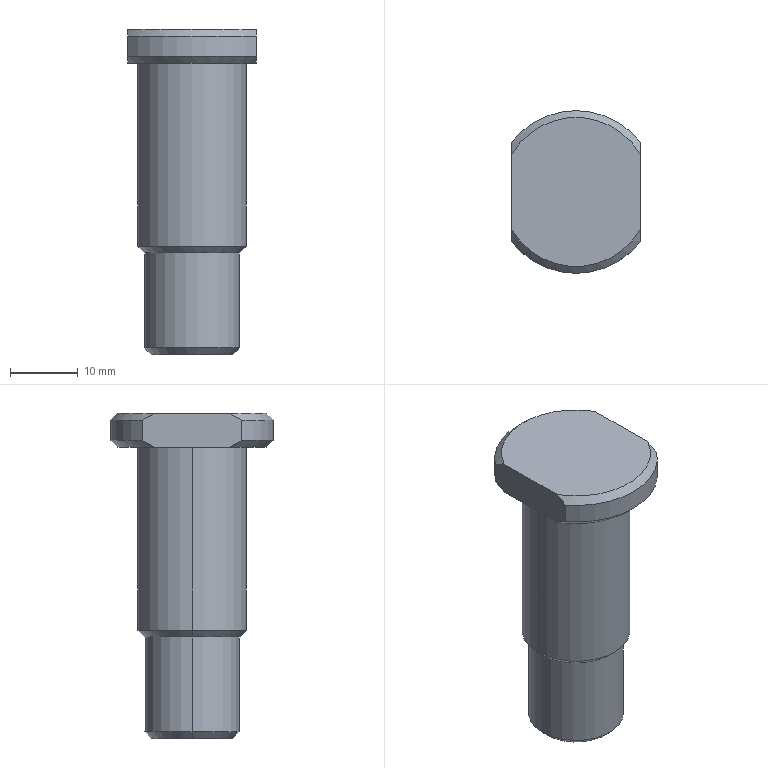Part | SolidWorks | features BaseBody 1 | 1 solid | 19 faces | box 19 x 24 x 48 mm | volume 9861 mm3 | cone 8 | cylinder 6 | plane 5 | commonest cylinder face diameters 14 x2 16 x2 24 x2
STEP:
#1=CARTESIAN_POINT('',(-6.,0.,0.));
#2=VERTEX_POINT('',#1);
#3=CARTESIAN_POINT('',(6.,0.,0.));
#4=VERTEX_POINT('',#3);
#5=CARTESIAN_POINT('',(0.,0.,0.));
#6=DIRECTION('',(0.,0.,-1.));
#7=DIRECTION('',(1.,0.,0.));
#8=AXIS2_PLACEMENT_3D('',#5,#6,#7);
#9=CIRCLE('',#8,6.);
#10=EDGE_CURVE('',#2,#4,#9,.T.);
#11=ORIENTED_EDGE('',*,*,#10,.F.);
#12=CARTESIAN_POINT('',(-7.,0.,1.));
#13=VERTEX_POINT('',#12);
#14=CARTESIAN_POINT('',(-7.,0.,1.));
#15=DIRECTION('',(-0.7071,0.,0.7071));
#16=VECTOR('',#15,1000.);
#17=LINE('',#14,#16);
#18=EDGE_CURVE('',#2,#13,#17,.T.);
#19=ORIENTED_EDGE('',*,*,#18,.T.);
#20=CARTESIAN_POINT('',(7.,0.,1.));
#21=VERTEX_POINT('',#20);
#22=CARTESIAN_POINT('',(0.,0.,1.));
#23=DIRECTION('',(0.,0.,1.));
#24=DIRECTION('',(1.,0.,0.));
#25=AXIS2_PLACEMENT_3D('',#22,#23,#24);
#26=CIRCLE('',#25,7.);
#27=EDGE_CURVE('',#21,#13,#26,.T.);
#28=ORIENTED_EDGE('',*,*,#27,.F.);
#29=CARTESIAN_POINT('',(7.,0.,1.));
#30=DIRECTION('',(0.7071,0.,0.7071));
#31=VECTOR('',#30,1000.);
#32=LINE('',#29,#31);
#33=EDGE_CURVE('',#4,#21,#32,.T.);
#34=ORIENTED_EDGE('',*,*,#33,.F.);
#35=EDGE_LOOP('',(#11,#19,#28,#34));
#36=FACE_OUTER_BOUND('',#35,.T.);
#37=CARTESIAN_POINT('',(0.,0.,1.));
#38=DIRECTION('',(0.,0.,1.));
#39=DIRECTION('',(1.,0.,0.));
#40=AXIS2_PLACEMENT_3D('',#37,#38,#39);
#41=CONICAL_SURFACE('',#40,7.,0.7854);
#42=ADVANCED_FACE('',(#36),#41,.T.);
#43=CARTESIAN_POINT('',(7.,0.,15.));
#44=VERTEX_POINT('',#43);
#45=CARTESIAN_POINT('',(-7.,0.,15.));
#46=VERTEX_POINT('',#45);
#47=CARTESIAN_POINT('',(0.,0.,15.));
#48=DIRECTION('',(0.,0.,1.));
#49=DIRECTION('',(1.,0.,0.));
#50=AXIS2_PLACEMENT_3D('',#47,#48,#49);
#51=CIRCLE('',#50,7.);
#52=EDGE_CURVE('',#44,#46,#51,.T.);
#53=ORIENTED_EDGE('',*,*,#52,.T.);
#54=CARTESIAN_POINT('',(-8.,0.,16.));
#55=VERTEX_POINT('',#54);
#56=CARTESIAN_POINT('',(-8.,0.,16.));
#57=DIRECTION('',(-0.7071,0.,0.7071));
#58=VECTOR('',#57,1000.);
#59=LINE('',#56,#58);
#60=EDGE_CURVE('',#46,#55,#59,.T.);
#61=ORIENTED_EDGE('',*,*,#60,.T.);
#62=CARTESIAN_POINT('',(8.,0.,16.));
#63=VERTEX_POINT('',#62);
#64=CARTESIAN_POINT('',(0.,0.,16.));
#65=DIRECTION('',(0.,0.,1.));
#66=DIRECTION('',(1.,0.,0.));
#67=AXIS2_PLACEMENT_3D('',#64,#65,#66);
#68=CIRCLE('',#67,8.);
#69=EDGE_CURVE('',#63,#55,#68,.T.);
#70=ORIENTED_EDGE('',*,*,#69,.F.);
#71=CARTESIAN_POINT('',(8.,0.,16.));
#72=DIRECTION('',(0.7071,0.,0.7071));
#73=VECTOR('',#72,1000.);
#74=LINE('',#71,#73);
#75=EDGE_CURVE('',#44,#63,#74,.T.);
#76=ORIENTED_EDGE('',*,*,#75,.F.);
#77=EDGE_LOOP('',(#53,#61,#70,#76));
#78=FACE_OUTER_BOUND('',#77,.T.);
#79=CARTESIAN_POINT('',(0.,0.,16.));
#80=DIRECTION('',(0.,0.,1.));
#81=DIRECTION('',(1.,0.,0.));
#82=AXIS2_PLACEMENT_3D('',#79,#80,#81);
#83=CONICAL_SURFACE('',#82,8.,0.7854);
#84=ADVANCED_FACE('',(#78),#83,.T.);
#85=CARTESIAN_POINT('',(8.,0.,43.));
#86=VERTEX_POINT('',#85);
#87=CARTESIAN_POINT('',(-8.,0.,43.));
#88=VERTEX_POINT('',#87);
#89=CARTESIAN_POINT('',(0.,0.,43.));
#90=DIRECTION('',(0.,0.,1.));
#91=DIRECTION('',(1.,0.,0.));
#92=AXIS2_PLACEMENT_3D('',#89,#90,#91);
#93=CIRCLE('',#92,8.);
#94=EDGE_CURVE('',#86,#88,#93,.T.);
#95=ORIENTED_EDGE('',*,*,#94,.F.);
#96=CARTESIAN_POINT('',(8.,0.,43.));
#97=DIRECTION('',(0.,0.,-1.));
#98=VECTOR('',#97,1000.);
#99=LINE('',#96,#98);
#100=EDGE_CURVE('',#86,#63,#99,.T.);
#101=ORIENTED_EDGE('',*,*,#100,.T.);
#102=ORIENTED_EDGE('',*,*,#69,.T.);
#103=CARTESIAN_POINT('',(-8.,0.,43.));
#104=DIRECTION('',(0.,0.,-1.));
#105=VECTOR('',#104,1000.);
#106=LINE('',#103,#105);
#107=EDGE_CURVE('',#88,#55,#106,.T.);
#108=ORIENTED_EDGE('',*,*,#107,.F.);
#109=EDGE_LOOP('',(#95,#101,#102,#108));
#110=FACE_OUTER_BOUND('',#109,.T.);
#111=CARTESIAN_POINT('',(0.,0.,43.));
#112=DIRECTION('',(0.,0.,-1.));
#113=DIRECTION('',(-1.,0.,0.));
#114=AXIS2_PLACEMENT_3D('',#111,#112,#113);
#115=CYLINDRICAL_SURFACE('',#114,8.);
#116=ADVANCED_FACE('',(#110),#115,.T.);
#117=ORIENTED_EDGE('',*,*,#52,.F.);
#118=CARTESIAN_POINT('',(7.,0.,15.));
#119=DIRECTION('',(0.,0.,-1.));
#120=VECTOR('',#119,1000.);
#121=LINE('',#118,#120);
#122=EDGE_CURVE('',#44,#21,#121,.T.);
#123=ORIENTED_EDGE('',*,*,#122,.T.);
#124=ORIENTED_EDGE('',*,*,#27,.T.);
#125=CARTESIAN_POINT('',(-7.,0.,15.));
#126=DIRECTION('',(0.,0.,-1.));
#127=VECTOR('',#126,1000.);
#128=LINE('',#125,#127);
#129=EDGE_CURVE('',#46,#13,#128,.T.);
#130=ORIENTED_EDGE('',*,*,#129,.F.);
#131=EDGE_LOOP('',(#117,#123,#124,#130));
#132=FACE_OUTER_BOUND('',#131,.T.);
#133=CARTESIAN_POINT('',(0.,0.,15.));
#134=DIRECTION('',(0.,0.,-1.));
#135=DIRECTION('',(-1.,0.,0.));
#136=AXIS2_PLACEMENT_3D('',#133,#134,#135);
#137=CYLINDRICAL_SURFACE('',#136,7.);
#138=ADVANCED_FACE('',(#132),#137,.T.);
#139=CARTESIAN_POINT('',(-9.5,-5.545,43.));
#140=VERTEX_POINT('',#139);
#141=CARTESIAN_POINT('',(-9.5,-7.331,44.));
#142=VERTEX_POINT('',#141);
#143=CARTESIAN_POINT('',(-9.5,-5.545,43.));
#144=CARTESIAN_POINT('',(-9.5,-6.4,43.431));
#145=CARTESIAN_POINT('',(-9.5,-7.331,44.));
#146=(BOUNDED_CURVE()B_SPLINE_CURVE(2,(#143,#144,#145),.UNSPECIFIED.,.F.,.F.)B_SPLINE_CURVE_WITH_KNOTS((3,3),(0.3475,0.5859),.UNSPECIFIED.)CURVE()GEOMETRIC_REPRESENTATION_ITEM()RATIONAL_B_SPLINE_CURVE((1.037,1.045,1.047))REPRESENTATION_ITEM(''));
#147=EDGE_CURVE('',#140,#142,#146,.T.);
#148=ORIENTED_EDGE('',*,*,#147,.F.);
#149=CARTESIAN_POINT('',(9.5,-5.545,43.));
#150=VERTEX_POINT('',#149);
#151=CARTESIAN_POINT('',(0.,0.,43.));
#152=DIRECTION('',(0.,0.,-1.));
#153=DIRECTION('',(1.,0.,0.));
#154=AXIS2_PLACEMENT_3D('',#151,#152,#153);
#155=CIRCLE('',#154,11.);
#156=EDGE_CURVE('',#150,#140,#155,.T.);
#157=ORIENTED_EDGE('',*,*,#156,.F.);
#158=CARTESIAN_POINT('',(9.5,-7.331,44.));
#159=VERTEX_POINT('',#158);
#160=CARTESIAN_POINT('',(9.5,-7.331,44.));
#161=CARTESIAN_POINT('',(9.5,-6.4,43.431));
#162=CARTESIAN_POINT('',(9.5,-5.545,43.));
#163=(BOUNDED_CURVE()B_SPLINE_CURVE(2,(#160,#161,#162),.UNSPECIFIED.,.F.,.F.)B_SPLINE_CURVE_WITH_KNOTS((3,3),(0.7213,0.9597),.UNSPECIFIED.)CURVE()GEOMETRIC_REPRESENTATION_ITEM()RATIONAL_B_SPLINE_CURVE((1.047,1.045,1.037))REPRESENTATION_ITEM(''));
#164=EDGE_CURVE('',#159,#150,#163,.T.);
#165=ORIENTED_EDGE('',*,*,#164,.F.);
#166=CARTESIAN_POINT('',(0.,0.,44.));
#167=DIRECTION('',(0.,0.,1.));
#168=DIRECTION('',(1.,0.,0.));
#169=AXIS2_PLACEMENT_3D('',#166,#167,#168);
#170=CIRCLE('',#169,12.);
#171=EDGE_CURVE('',#142,#159,#170,.T.);
#172=ORIENTED_EDGE('',*,*,#171,.F.);
#173=EDGE_LOOP('',(#148,#157,#165,#172));
#174=FACE_OUTER_BOUND('',#173,.T.);
#175=CARTESIAN_POINT('',(0.,0.,44.));
#176=DIRECTION('',(0.,0.,1.));
#177=DIRECTION('',(1.,0.,0.));
#178=AXIS2_PLACEMENT_3D('',#175,#176,#177);
#179=CONICAL_SURFACE('',#178,12.,0.7854);
#180=ADVANCED_FACE('',(#174),#179,.T.);
#181=CARTESIAN_POINT('',(9.5,5.545,43.));
#182=VERTEX_POINT('',#181);
#183=CARTESIAN_POINT('',(9.5,7.331,44.));
#184=VERTEX_POINT('',#183);
#185=CARTESIAN_POINT('',(9.5,5.545,43.));
#186=CARTESIAN_POINT('',(9.5,6.4,43.431));
#187=CARTESIAN_POINT('',(9.5,7.331,44.));
#188=(BOUNDED_CURVE()B_SPLINE_CURVE(2,(#185,#186,#187),.UNSPECIFIED.,.F.,.F.)B_SPLINE_CURVE_WITH_KNOTS((3,3),(0.3475,0.5859),.UNSPECIFIED.)CURVE()GEOMETRIC_REPRESENTATION_ITEM()RATIONAL_B_SPLINE_CURVE((1.037,1.045,1.047))REPRESENTATION_ITEM(''));
#189=EDGE_CURVE('',#182,#184,#188,.T.);
#190=ORIENTED_EDGE('',*,*,#189,.F.);
#191=CARTESIAN_POINT('',(-9.5,5.545,43.));
#192=VERTEX_POINT('',#191);
#193=CARTESIAN_POINT('',(0.,0.,43.));
#194=DIRECTION('',(0.,0.,-1.));
#195=DIRECTION('',(1.,0.,0.));
#196=AXIS2_PLACEMENT_3D('',#193,#194,#195);
#197=CIRCLE('',#196,11.);
#198=EDGE_CURVE('',#192,#182,#197,.T.);
#199=ORIENTED_EDGE('',*,*,#198,.F.);
#200=CARTESIAN_POINT('',(-9.5,7.331,44.));
#201=VERTEX_POINT('',#200);
#202=CARTESIAN_POINT('',(-9.5,7.331,44.));
#203=CARTESIAN_POINT('',(-9.5,6.4,43.431));
#204=CARTESIAN_POINT('',(-9.5,5.545,43.));
#205=(BOUNDED_CURVE()B_SPLINE_CURVE(2,(#202,#203,#204),.UNSPECIFIED.,.F.,.F.)B_SPLINE_CURVE_WITH_KNOTS((3,3),(0.7213,0.9597),.UNSPECIFIED.)CURVE()GEOMETRIC_REPRESENTATION_ITEM()RATIONAL_B_SPLINE_CURVE((1.047,1.045,1.037))REPRESENTATION_ITEM(''));
#206=EDGE_CURVE('',#201,#192,#205,.T.);
#207=ORIENTED_EDGE('',*,*,#206,.F.);
#208=CARTESIAN_POINT('',(0.,0.,44.));
#209=DIRECTION('',(0.,0.,1.));
#210=DIRECTION('',(1.,0.,0.));
#211=AXIS2_PLACEMENT_3D('',#208,#209,#210);
#212=CIRCLE('',#211,12.);
#213=EDGE_CURVE('',#184,#201,#212,.T.);
#214=ORIENTED_EDGE('',*,*,#213,.F.);
#215=EDGE_LOOP('',(#190,#199,#207,#214));
#216=FACE_OUTER_BOUND('',#215,.T.);
#217=CARTESIAN_POINT('',(0.,0.,44.));
#218=DIRECTION('',(0.,0.,1.));
#219=DIRECTION('',(1.,0.,0.));
#220=AXIS2_PLACEMENT_3D('',#217,#218,#219);
#221=CONICAL_SURFACE('',#220,12.,0.7854);
#222=ADVANCED_FACE('',(#216),#221,.T.);
#223=CARTESIAN_POINT('',(-9.5,-7.331,47.));
#224=VERTEX_POINT('',#223);
#225=CARTESIAN_POINT('',(-9.5,-5.545,48.));
#226=VERTEX_POINT('',#225);
#227=CARTESIAN_POINT('',(-9.5,-7.331,47.));
#228=CARTESIAN_POINT('',(-9.5,-6.4,47.569));
#229=CARTESIAN_POINT('',(-9.5,-5.545,48.));
#230=(BOUNDED_CURVE()B_SPLINE_CURVE(2,(#227,#228,#229),.UNSPECIFIED.,.F.,.T.)B_SPLINE_CURVE_WITH_KNOTS((3,3),(0.7213,0.9597),.UNSPECIFIED.)CURVE()GEOMETRIC_REPRESENTATION_ITEM()RATIONAL_B_SPLINE_CURVE((1.047,1.045,1.037))REPRESENTATION_ITEM(''));
#231=EDGE_CURVE('',#224,#226,#230,.T.);
#232=ORIENTED_EDGE('',*,*,#231,.F.);
#233=CARTESIAN_POINT('',(9.5,-7.331,47.));
#234=VERTEX_POINT('',#233);
#235=CARTESIAN_POINT('',(0.,0.,47.));
#236=DIRECTION('',(0.,0.,-1.));
#237=DIRECTION('',(1.,0.,0.));
#238=AXIS2_PLACEMENT_3D('',#235,#236,#237);
#239=CIRCLE('',#238,12.);
#240=EDGE_CURVE('',#234,#224,#239,.T.);
#241=ORIENTED_EDGE('',*,*,#240,.F.);
#242=CARTESIAN_POINT('',(9.5,-5.545,48.));
#243=VERTEX_POINT('',#242);
#244=CARTESIAN_POINT('',(9.5,-5.545,48.));
#245=CARTESIAN_POINT('',(9.5,-6.4,47.569));
#246=CARTESIAN_POINT('',(9.5,-7.331,47.));
#247=(BOUNDED_CURVE()B_SPLINE_CURVE(2,(#244,#245,#246),.UNSPECIFIED.,.F.,.T.)B_SPLINE_CURVE_WITH_KNOTS((3,3),(0.3475,0.5859),.UNSPECIFIED.)CURVE()GEOMETRIC_REPRESENTATION_ITEM()RATIONAL_B_SPLINE_CURVE((1.037,1.045,1.047))REPRESENTATION_ITEM(''));
#248=EDGE_CURVE('',#243,#234,#247,.T.);
#249=ORIENTED_EDGE('',*,*,#248,.F.);
#250=CARTESIAN_POINT('',(0.,0.,48.));
#251=DIRECTION('',(0.,0.,1.));
#252=DIRECTION('',(1.,0.,0.));
#253=AXIS2_PLACEMENT_3D('',#250,#251,#252);
#254=CIRCLE('',#253,11.);
#255=EDGE_CURVE('',#226,#243,#254,.T.);
#256=ORIENTED_EDGE('',*,*,#255,.F.);
#257=EDGE_LOOP('',(#232,#241,#249,#256));
#258=FACE_OUTER_BOUND('',#257,.T.);
#259=CARTESIAN_POINT('',(0.,0.,48.));
#260=DIRECTION('',(0.,0.,-1.));
#261=DIRECTION('',(-1.,0.,0.));
#262=AXIS2_PLACEMENT_3D('',#259,#260,#261);
#263=CONICAL_SURFACE('',#262,11.,0.7854);
#264=ADVANCED_FACE('',(#258),#263,.T.);
#265=CARTESIAN_POINT('',(9.5,7.331,47.));
#266=VERTEX_POINT('',#265);
#267=CARTESIAN_POINT('',(9.5,5.545,48.));
#268=VERTEX_POINT('',#267);
#269=CARTESIAN_POINT('',(9.5,7.331,47.));
#270=CARTESIAN_POINT('',(9.5,6.4,47.569));
#271=CARTESIAN_POINT('',(9.5,5.545,48.));
#272=(BOUNDED_CURVE()B_SPLINE_CURVE(2,(#269,#270,#271),.UNSPECIFIED.,.F.,.F.)B_SPLINE_CURVE_WITH_KNOTS((3,3),(0.7213,0.9597),.UNSPECIFIED.)CURVE()GEOMETRIC_REPRESENTATION_ITEM()RATIONAL_B_SPLINE_CURVE((1.047,1.045,1.037))REPRESENTATION_ITEM(''));
#273=EDGE_CURVE('',#266,#268,#272,.T.);
#274=ORIENTED_EDGE('',*,*,#273,.F.);
#275=CARTESIAN_POINT('',(-9.5,7.331,47.));
#276=VERTEX_POINT('',#275);
#277=CARTESIAN_POINT('',(0.,0.,47.));
#278=DIRECTION('',(0.,0.,-1.));
#279=DIRECTION('',(1.,0.,0.));
#280=AXIS2_PLACEMENT_3D('',#277,#278,#279);
#281=CIRCLE('',#280,12.);
#282=EDGE_CURVE('',#276,#266,#281,.T.);
#283=ORIENTED_EDGE('',*,*,#282,.F.);
#284=CARTESIAN_POINT('',(-9.5,5.545,48.));
#285=VERTEX_POINT('',#284);
#286=CARTESIAN_POINT('',(-9.5,5.545,48.));
#287=CARTESIAN_POINT('',(-9.5,6.4,47.569));
#288=CARTESIAN_POINT('',(-9.5,7.331,47.));
#289=(BOUNDED_CURVE()B_SPLINE_CURVE(2,(#286,#287,#288),.UNSPECIFIED.,.F.,.T.)B_SPLINE_CURVE_WITH_KNOTS((3,3),(0.3475,0.5859),.UNSPECIFIED.)CURVE()GEOMETRIC_REPRESENTATION_ITEM()RATIONAL_B_SPLINE_CURVE((1.037,1.045,1.047))REPRESENTATION_ITEM(''));
#290=EDGE_CURVE('',#285,#276,#289,.T.);
#291=ORIENTED_EDGE('',*,*,#290,.F.);
#292=CARTESIAN_POINT('',(0.,0.,48.));
#293=DIRECTION('',(0.,0.,1.));
#294=DIRECTION('',(1.,0.,0.));
#295=AXIS2_PLACEMENT_3D('',#292,#293,#294);
#296=CIRCLE('',#295,11.);
#297=EDGE_CURVE('',#268,#285,#296,.T.);
#298=ORIENTED_EDGE('',*,*,#297,.F.);
#299=EDGE_LOOP('',(#274,#283,#291,#298));
#300=FACE_OUTER_BOUND('',#299,.T.);
#301=CARTESIAN_POINT('',(0.,0.,48.));
#302=DIRECTION('',(0.,0.,-1.));
#303=DIRECTION('',(-1.,0.,0.));
#304=AXIS2_PLACEMENT_3D('',#301,#302,#303);
#305=CONICAL_SURFACE('',#304,11.,0.7854);
#306=ADVANCED_FACE('',(#300),#305,.T.);
#307=CARTESIAN_POINT('',(-9.5,17.5,48.));
#308=DIRECTION('',(0.,-1.,0.));
#309=VECTOR('',#308,1000.);
#310=LINE('',#307,#309);
#311=EDGE_CURVE('',#285,#226,#310,.T.);
#312=ORIENTED_EDGE('',*,*,#311,.F.);
#313=ORIENTED_EDGE('',*,*,#290,.T.);
#314=CARTESIAN_POINT('',(-9.5,7.331,48.));
#315=DIRECTION('',(0.,0.,-1.));
#316=VECTOR('',#315,1000.);
#317=LINE('',#314,#316);
#318=EDGE_CURVE('',#276,#201,#317,.T.);
#319=ORIENTED_EDGE('',*,*,#318,.T.);
#320=ORIENTED_EDGE('',*,*,#206,.T.);
#321=CARTESIAN_POINT('',(-9.5,0.,43.));
#322=DIRECTION('',(0.,-1.,0.));
#323=VECTOR('',#322,1000.);
#324=LINE('',#321,#323);
#325=EDGE_CURVE('',#192,#140,#324,.T.);
#326=ORIENTED_EDGE('',*,*,#325,.T.);
#327=ORIENTED_EDGE('',*,*,#147,.T.);
#328=CARTESIAN_POINT('',(-9.5,-7.331,48.));
#329=DIRECTION('',(0.,0.,1.));
#330=VECTOR('',#329,1000.);
#331=LINE('',#328,#330);
#332=EDGE_CURVE('',#142,#224,#331,.T.);
#333=ORIENTED_EDGE('',*,*,#332,.T.);
#334=ORIENTED_EDGE('',*,*,#231,.T.);
#335=EDGE_LOOP('',(#312,#313,#319,#320,#326,#327,#333,#334));
#336=FACE_OUTER_BOUND('',#335,.T.);
#337=CARTESIAN_POINT('',(-9.5,17.5,43.));
#338=DIRECTION('',(-1.,0.,0.));
#339=DIRECTION('',(0.,1.,0.));
#340=AXIS2_PLACEMENT_3D('',#337,#338,#339);
#341=PLANE('',#340);
#342=ADVANCED_FACE('',(#336),#341,.T.);
#343=CARTESIAN_POINT('',(9.5,7.331,48.));
#344=DIRECTION('',(0.,0.,1.));
#345=VECTOR('',#344,1000.);
#346=LINE('',#343,#345);
#347=EDGE_CURVE('',#184,#266,#346,.T.);
#348=ORIENTED_EDGE('',*,*,#347,.T.);
#349=ORIENTED_EDGE('',*,*,#273,.T.);
#350=CARTESIAN_POINT('',(9.5,17.5,48.));
#351=DIRECTION('',(0.,1.,0.));
#352=VECTOR('',#351,1000.);
#353=LINE('',#350,#352);
#354=EDGE_CURVE('',#243,#268,#353,.T.);
#355=ORIENTED_EDGE('',*,*,#354,.F.);
#356=ORIENTED_EDGE('',*,*,#248,.T.);
#357=CARTESIAN_POINT('',(9.5,-7.331,48.));
#358=DIRECTION('',(0.,0.,-1.));
#359=VECTOR('',#358,1000.);
#360=LINE('',#357,#359);
#361=EDGE_CURVE('',#234,#159,#360,.T.);
#362=ORIENTED_EDGE('',*,*,#361,.T.);
#363=ORIENTED_EDGE('',*,*,#164,.T.);
#364=CARTESIAN_POINT('',(9.5,0.,43.));
#365=DIRECTION('',(0.,1.,0.));
#366=VECTOR('',#365,1000.);
#367=LINE('',#364,#366);
#368=EDGE_CURVE('',#150,#182,#367,.T.);
#369=ORIENTED_EDGE('',*,*,#368,.T.);
#370=ORIENTED_EDGE('',*,*,#189,.T.);
#371=EDGE_LOOP('',(#348,#349,#355,#356,#362,#363,#369,#370));
#372=FACE_OUTER_BOUND('',#371,.T.);
#373=CARTESIAN_POINT('',(9.5,17.5,43.));
#374=DIRECTION('',(1.,0.,0.));
#375=DIRECTION('',(0.,1.,0.));
#376=AXIS2_PLACEMENT_3D('',#373,#374,#375);
#377=PLANE('',#376);
#378=ADVANCED_FACE('',(#372),#377,.T.);
#379=CARTESIAN_POINT('',(0.,0.,0.));
#380=DIRECTION('',(0.,0.,-1.));
#381=DIRECTION('',(1.,0.,0.));
#382=AXIS2_PLACEMENT_3D('',#379,#380,#381);
#383=CIRCLE('',#382,6.);
#384=EDGE_CURVE('',#4,#2,#383,.T.);
#385=ORIENTED_EDGE('',*,*,#384,.T.);
#386=ORIENTED_EDGE('',*,*,#10,.T.);
#387=EDGE_LOOP('',(#385,#386));
#388=FACE_OUTER_BOUND('',#387,.T.);
#389=CARTESIAN_POINT('',(0.,0.,0.));
#390=DIRECTION('',(0.,0.,1.));
#391=DIRECTION('',(1.,0.,0.));
#392=AXIS2_PLACEMENT_3D('',#389,#390,#391);
#393=PLANE('',#392);
#394=ADVANCED_FACE('',(#388),#393,.F.);
#395=CARTESIAN_POINT('',(0.,0.,43.));
#396=DIRECTION('',(0.,0.,1.));
#397=DIRECTION('',(1.,0.,0.));
#398=AXIS2_PLACEMENT_3D('',#395,#396,#397);
#399=CIRCLE('',#398,8.);
#400=EDGE_CURVE('',#88,#86,#399,.T.);
#401=ORIENTED_EDGE('',*,*,#400,.T.);
#402=ORIENTED_EDGE('',*,*,#94,.T.);
#403=EDGE_LOOP('',(#401,#402));
#404=FACE_BOUND('',#403,.T.);
#405=ORIENTED_EDGE('',*,*,#325,.F.);
#406=ORIENTED_EDGE('',*,*,#198,.T.);
#407=ORIENTED_EDGE('',*,*,#368,.F.);
#408=ORIENTED_EDGE('',*,*,#156,.T.);
#409=EDGE_LOOP('',(#405,#406,#407,#408));
#410=FACE_OUTER_BOUND('',#409,.T.);
#411=CARTESIAN_POINT('',(0.,0.,43.));
#412=DIRECTION('',(0.,0.,1.));
#413=DIRECTION('',(1.,0.,0.));
#414=AXIS2_PLACEMENT_3D('',#411,#412,#413);
#415=PLANE('',#414);
#416=ADVANCED_FACE('',(#404,#410),#415,.F.);
#417=ORIENTED_EDGE('',*,*,#354,.T.);
#418=ORIENTED_EDGE('',*,*,#297,.T.);
#419=ORIENTED_EDGE('',*,*,#311,.T.);
#420=ORIENTED_EDGE('',*,*,#255,.T.);
#421=EDGE_LOOP('',(#417,#418,#419,#420));
#422=FACE_OUTER_BOUND('',#421,.T.);
#423=CARTESIAN_POINT('',(0.,0.,48.));
#424=DIRECTION('',(0.,0.,1.));
#425=DIRECTION('',(1.,0.,0.));
#426=AXIS2_PLACEMENT_3D('',#423,#424,#425);
#427=PLANE('',#426);
#428=ADVANCED_FACE('',(#422),#427,.T.);
#429=ORIENTED_EDGE('',*,*,#361,.F.);
#430=ORIENTED_EDGE('',*,*,#240,.T.);
#431=ORIENTED_EDGE('',*,*,#332,.F.);
#432=ORIENTED_EDGE('',*,*,#171,.T.);
#433=EDGE_LOOP('',(#429,#430,#431,#432));
#434=FACE_OUTER_BOUND('',#433,.T.);
#435=CARTESIAN_POINT('',(0.,0.,48.));
#436=DIRECTION('',(0.,0.,-1.));
#437=DIRECTION('',(-1.,0.,0.));
#438=AXIS2_PLACEMENT_3D('',#435,#436,#437);
#439=CYLINDRICAL_SURFACE('',#438,12.);
#440=ADVANCED_FACE('',(#434),#439,.T.);
#441=ORIENTED_EDGE('',*,*,#318,.F.);
#442=ORIENTED_EDGE('',*,*,#282,.T.);
#443=ORIENTED_EDGE('',*,*,#347,.F.);
#444=ORIENTED_EDGE('',*,*,#213,.T.);
#445=EDGE_LOOP('',(#441,#442,#443,#444));
#446=FACE_OUTER_BOUND('',#445,.T.);
#447=CARTESIAN_POINT('',(0.,0.,48.));
#448=DIRECTION('',(0.,0.,-1.));
#449=DIRECTION('',(-1.,0.,0.));
#450=AXIS2_PLACEMENT_3D('',#447,#448,#449);
#451=CYLINDRICAL_SURFACE('',#450,12.);
#452=ADVANCED_FACE('',(#446),#451,.T.);
#453=ORIENTED_EDGE('',*,*,#122,.F.);
#454=CARTESIAN_POINT('',(0.,0.,15.));
#455=DIRECTION('',(0.,0.,1.));
#456=DIRECTION('',(1.,0.,0.));
#457=AXIS2_PLACEMENT_3D('',#454,#455,#456);
#458=CIRCLE('',#457,7.);
#459=EDGE_CURVE('',#46,#44,#458,.T.);
#460=ORIENTED_EDGE('',*,*,#459,.F.);
#461=ORIENTED_EDGE('',*,*,#129,.T.);
#462=CARTESIAN_POINT('',(0.,0.,1.));
#463=DIRECTION('',(0.,0.,1.));
#464=DIRECTION('',(1.,0.,0.));
#465=AXIS2_PLACEMENT_3D('',#462,#463,#464);
#466=CIRCLE('',#465,7.);
#467=EDGE_CURVE('',#13,#21,#466,.T.);
#468=ORIENTED_EDGE('',*,*,#467,.T.);
#469=EDGE_LOOP('',(#453,#460,#461,#468));
#470=FACE_OUTER_BOUND('',#469,.T.);
#471=CARTESIAN_POINT('',(0.,0.,15.));
#472=DIRECTION('',(0.,0.,-1.));
#473=DIRECTION('',(-1.,0.,0.));
#474=AXIS2_PLACEMENT_3D('',#471,#472,#473);
#475=CYLINDRICAL_SURFACE('',#474,7.);
#476=ADVANCED_FACE('',(#470),#475,.T.);
#477=ORIENTED_EDGE('',*,*,#100,.F.);
#478=ORIENTED_EDGE('',*,*,#400,.F.);
#479=ORIENTED_EDGE('',*,*,#107,.T.);
#480=CARTESIAN_POINT('',(0.,0.,16.));
#481=DIRECTION('',(0.,0.,1.));
#482=DIRECTION('',(1.,0.,0.));
#483=AXIS2_PLACEMENT_3D('',#480,#481,#482);
#484=CIRCLE('',#483,8.);
#485=EDGE_CURVE('',#55,#63,#484,.T.);
#486=ORIENTED_EDGE('',*,*,#485,.T.);
#487=EDGE_LOOP('',(#477,#478,#479,#486));
#488=FACE_OUTER_BOUND('',#487,.T.);
#489=CARTESIAN_POINT('',(0.,0.,43.));
#490=DIRECTION('',(0.,0.,-1.));
#491=DIRECTION('',(-1.,0.,0.));
#492=AXIS2_PLACEMENT_3D('',#489,#490,#491);
#493=CYLINDRICAL_SURFACE('',#492,8.);
#494=ADVANCED_FACE('',(#488),#493,.T.);
#495=ORIENTED_EDGE('',*,*,#60,.F.);
#496=ORIENTED_EDGE('',*,*,#459,.T.);
#497=ORIENTED_EDGE('',*,*,#75,.T.);
#498=ORIENTED_EDGE('',*,*,#485,.F.);
#499=EDGE_LOOP('',(#495,#496,#497,#498));
#500=FACE_OUTER_BOUND('',#499,.T.);
#501=CARTESIAN_POINT('',(0.,0.,16.));
#502=DIRECTION('',(0.,0.,1.));
#503=DIRECTION('',(1.,0.,0.));
#504=AXIS2_PLACEMENT_3D('',#501,#502,#503);
#505=CONICAL_SURFACE('',#504,8.,0.7854);
#506=ADVANCED_FACE('',(#500),#505,.T.);
#507=ORIENTED_EDGE('',*,*,#18,.F.);
#508=ORIENTED_EDGE('',*,*,#384,.F.);
#509=ORIENTED_EDGE('',*,*,#33,.T.);
#510=ORIENTED_EDGE('',*,*,#467,.F.);
#511=EDGE_LOOP('',(#507,#508,#509,#510));
#512=FACE_OUTER_BOUND('',#511,.T.);
#513=CARTESIAN_POINT('',(0.,0.,1.));
#514=DIRECTION('',(0.,0.,1.));
#515=DIRECTION('',(1.,0.,0.));
#516=AXIS2_PLACEMENT_3D('',#513,#514,#515);
#517=CONICAL_SURFACE('',#516,7.,0.7854);
#518=ADVANCED_FACE('',(#512),#517,.T.);
#519=CLOSED_SHELL('',(#42,#84,#116,#138,#180,#222,#264,#306,#342,#378,#394,#416,#428,#440,#452,#476,#494,#506,#518));
#520=MANIFOLD_SOLID_BREP('',#519);
#521=CARTESIAN_POINT('',(0.,0.,0.));
#522=DIRECTION('',(0.,0.,1.));
#523=DIRECTION('',(1.,0.,0.));
#524=AXIS2_PLACEMENT_3D('',#521,#522,#523);
#525=(LENGTH_UNIT()NAMED_UNIT(*)SI_UNIT(.MILLI.,.METRE.));
#526=UNCERTAINTY_MEASURE_WITH_UNIT(LENGTH_MEASURE(0.00001),#525,'','');
#527=(NAMED_UNIT(*)PLANE_ANGLE_UNIT()SI_UNIT($,.RADIAN.));
#528=(NAMED_UNIT(*)SI_UNIT($,.STERADIAN.)SOLID_ANGLE_UNIT());
#529=(GEOMETRIC_REPRESENTATION_CONTEXT(3)GLOBAL_UNCERTAINTY_ASSIGNED_CONTEXT((#526))GLOBAL_UNIT_ASSIGNED_CONTEXT((#525,#527,#528))REPRESENTATION_CONTEXT('',''));
#530=ADVANCED_BREP_SHAPE_REPRESENTATION('',(#520,#524),#529);